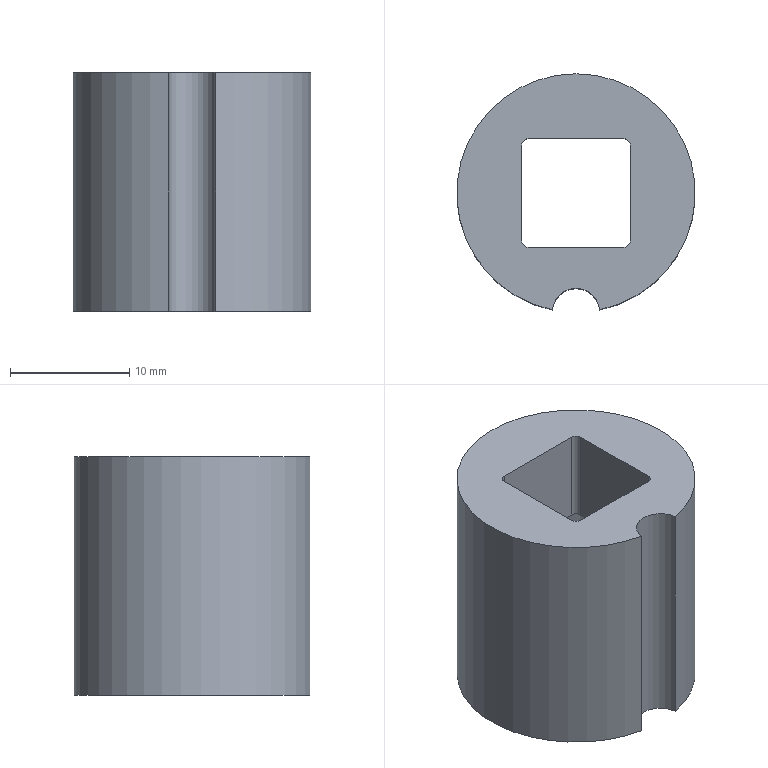Part | NX | features solid 2 | 1 solid | 14 faces | box 20 x 19.8 x 20 mm | volume 4006 mm3 | plane 7 | cylinder 7 | commonest cylinder face diameters 1.1 x4 4 x1 12.6 x1 20 x1
STEP:
#1=CARTESIAN_POINT('',(-513.119,-116.624,24.));
#2=VERTEX_POINT('',#1);
#3=CARTESIAN_POINT('',(-517.099,-116.624,24.));
#4=VERTEX_POINT('',#3);
#5=CARTESIAN_POINT('',(-515.109,-106.824,24.));
#6=DIRECTION('',(0.,0.,1.));
#7=DIRECTION('',(0.,-1.,0.));
#8=AXIS2_PLACEMENT_3D('',#5,#6,#7);
#9=CIRCLE('',#8,10.);
#10=EDGE_CURVE('',#2,#4,#9,.T.);
#11=ORIENTED_EDGE('',*,*,#10,.F.);
#12=CARTESIAN_POINT('',(-515.109,-116.824,24.));
#13=DIRECTION('',(0.,0.,1.));
#14=DIRECTION('',(0.,-1.,0.));
#15=AXIS2_PLACEMENT_3D('',#12,#13,#14);
#16=CIRCLE('',#15,2.);
#17=EDGE_CURVE('',#2,#4,#16,.T.);
#18=ORIENTED_EDGE('',*,*,#17,.T.);
#19=EDGE_LOOP('',(#11,#18));
#20=FACE_BOUND('',#19,.T.);
#21=CARTESIAN_POINT('',(-515.109,-113.124,24.));
#22=VERTEX_POINT('',#21);
#23=CARTESIAN_POINT('',(-515.109,-106.824,24.));
#24=DIRECTION('',(0.,0.,1.));
#25=DIRECTION('',(0.,-1.,0.));
#26=AXIS2_PLACEMENT_3D('',#23,#24,#25);
#27=CIRCLE('',#26,6.3);
#28=EDGE_CURVE('',#22,#22,#27,.T.);
#29=ORIENTED_EDGE('',*,*,#28,.T.);
#30=EDGE_LOOP('',(#29));
#31=FACE_BOUND('',#30,.T.);
#32=CARTESIAN_POINT('',(-515.109,-106.824,24.));
#33=DIRECTION('',(0.,0.,1.));
#34=DIRECTION('',(0.,-1.,0.));
#35=AXIS2_PLACEMENT_3D('',#32,#33,#34);
#36=PLANE('',#35);
#37=ADVANCED_FACE('',(#20,#31),#36,.F.);
#38=ORIENTED_EDGE('',*,*,#28,.F.);
#39=EDGE_LOOP('',(#38));
#40=FACE_BOUND('',#39,.T.);
#41=CARTESIAN_POINT('',(-515.109,-113.124,36.));
#42=VERTEX_POINT('',#41);
#43=CARTESIAN_POINT('',(-515.109,-106.824,36.));
#44=DIRECTION('',(0.,0.,1.));
#45=DIRECTION('',(0.,-1.,0.));
#46=AXIS2_PLACEMENT_3D('',#43,#44,#45);
#47=CIRCLE('',#46,6.3);
#48=EDGE_CURVE('',#42,#42,#47,.T.);
#49=ORIENTED_EDGE('',*,*,#48,.T.);
#50=EDGE_LOOP('',(#49));
#51=FACE_BOUND('',#50,.T.);
#52=CARTESIAN_POINT('',(-515.109,-106.824,24.));
#53=DIRECTION('',(0.,0.,1.));
#54=DIRECTION('',(0.,-1.,0.));
#55=AXIS2_PLACEMENT_3D('',#52,#53,#54);
#56=CYLINDRICAL_SURFACE('',#55,6.3);
#57=ADVANCED_FACE('',(#40,#51),#56,.F.);
#58=ORIENTED_EDGE('',*,*,#48,.F.);
#59=EDGE_LOOP('',(#58));
#60=FACE_BOUND('',#59,.T.);
#61=CARTESIAN_POINT('',(-510.559,-110.824,36.));
#62=VERTEX_POINT('',#61);
#63=CARTESIAN_POINT('',(-510.559,-102.824,36.));
#64=VERTEX_POINT('',#63);
#65=CARTESIAN_POINT('',(-510.559,-106.824,36.));
#66=DIRECTION('',(0.,1.,0.));
#67=VECTOR('',#66,1000.);
#68=LINE('',#65,#67);
#69=EDGE_CURVE('',#62,#64,#68,.T.);
#70=ORIENTED_EDGE('',*,*,#69,.T.);
#71=CARTESIAN_POINT('',(-511.109,-102.274,36.));
#72=VERTEX_POINT('',#71);
#73=CARTESIAN_POINT('',(-511.109,-102.824,36.));
#74=DIRECTION('',(0.,0.,1.));
#75=DIRECTION('',(0.,-1.,0.));
#76=AXIS2_PLACEMENT_3D('',#73,#74,#75);
#77=CIRCLE('',#76,0.55);
#78=EDGE_CURVE('',#64,#72,#77,.T.);
#79=ORIENTED_EDGE('',*,*,#78,.T.);
#80=CARTESIAN_POINT('',(-519.109,-102.274,36.));
#81=VERTEX_POINT('',#80);
#82=CARTESIAN_POINT('',(-515.109,-102.274,36.));
#83=DIRECTION('',(-1.,0.,0.));
#84=VECTOR('',#83,1000.);
#85=LINE('',#82,#84);
#86=EDGE_CURVE('',#72,#81,#85,.T.);
#87=ORIENTED_EDGE('',*,*,#86,.T.);
#88=CARTESIAN_POINT('',(-519.659,-102.824,36.));
#89=VERTEX_POINT('',#88);
#90=CARTESIAN_POINT('',(-519.109,-102.824,36.));
#91=DIRECTION('',(0.,0.,1.));
#92=DIRECTION('',(0.,-1.,0.));
#93=AXIS2_PLACEMENT_3D('',#90,#91,#92);
#94=CIRCLE('',#93,0.55);
#95=EDGE_CURVE('',#81,#89,#94,.T.);
#96=ORIENTED_EDGE('',*,*,#95,.T.);
#97=CARTESIAN_POINT('',(-519.659,-110.824,36.));
#98=VERTEX_POINT('',#97);
#99=CARTESIAN_POINT('',(-519.659,-106.824,36.));
#100=DIRECTION('',(0.,-1.,0.));
#101=VECTOR('',#100,1000.);
#102=LINE('',#99,#101);
#103=EDGE_CURVE('',#89,#98,#102,.T.);
#104=ORIENTED_EDGE('',*,*,#103,.T.);
#105=CARTESIAN_POINT('',(-519.109,-111.374,36.));
#106=VERTEX_POINT('',#105);
#107=CARTESIAN_POINT('',(-519.109,-110.824,36.));
#108=DIRECTION('',(0.,0.,1.));
#109=DIRECTION('',(0.,-1.,0.));
#110=AXIS2_PLACEMENT_3D('',#107,#108,#109);
#111=CIRCLE('',#110,0.55);
#112=EDGE_CURVE('',#98,#106,#111,.T.);
#113=ORIENTED_EDGE('',*,*,#112,.T.);
#114=CARTESIAN_POINT('',(-511.109,-111.374,36.));
#115=VERTEX_POINT('',#114);
#116=CARTESIAN_POINT('',(-515.109,-111.374,36.));
#117=DIRECTION('',(-1.,0.,0.));
#118=VECTOR('',#117,1000.);
#119=LINE('',#116,#118);
#120=EDGE_CURVE('',#115,#106,#119,.T.);
#121=ORIENTED_EDGE('',*,*,#120,.F.);
#122=CARTESIAN_POINT('',(-511.109,-110.824,36.));
#123=DIRECTION('',(0.,0.,1.));
#124=DIRECTION('',(0.,-1.,0.));
#125=AXIS2_PLACEMENT_3D('',#122,#123,#124);
#126=CIRCLE('',#125,0.55);
#127=EDGE_CURVE('',#115,#62,#126,.T.);
#128=ORIENTED_EDGE('',*,*,#127,.T.);
#129=EDGE_LOOP('',(#70,#79,#87,#96,#104,#113,#121,#128));
#130=FACE_BOUND('',#129,.T.);
#131=CARTESIAN_POINT('',(-515.109,-106.824,36.));
#132=DIRECTION('',(0.,0.,1.));
#133=DIRECTION('',(0.,-1.,0.));
#134=AXIS2_PLACEMENT_3D('',#131,#132,#133);
#135=PLANE('',#134);
#136=ADVANCED_FACE('',(#60,#130),#135,.F.);
#137=CARTESIAN_POINT('',(-513.119,-116.624,44.));
#138=VERTEX_POINT('',#137);
#139=CARTESIAN_POINT('',(-513.119,-116.624,34.));
#140=DIRECTION('',(0.,0.,1.));
#141=VECTOR('',#140,1000.);
#142=LINE('',#139,#141);
#143=EDGE_CURVE('',#2,#138,#142,.T.);
#144=ORIENTED_EDGE('',*,*,#143,.F.);
#145=ORIENTED_EDGE('',*,*,#10,.T.);
#146=CARTESIAN_POINT('',(-517.099,-116.624,44.));
#147=VERTEX_POINT('',#146);
#148=CARTESIAN_POINT('',(-517.099,-116.624,34.));
#149=DIRECTION('',(0.,0.,1.));
#150=VECTOR('',#149,1000.);
#151=LINE('',#148,#150);
#152=EDGE_CURVE('',#147,#4,#151,.F.);
#153=ORIENTED_EDGE('',*,*,#152,.F.);
#154=CARTESIAN_POINT('',(-515.109,-106.824,44.));
#155=DIRECTION('',(0.,0.,1.));
#156=DIRECTION('',(0.,-1.,0.));
#157=AXIS2_PLACEMENT_3D('',#154,#155,#156);
#158=CIRCLE('',#157,10.);
#159=EDGE_CURVE('',#138,#147,#158,.T.);
#160=ORIENTED_EDGE('',*,*,#159,.F.);
#161=EDGE_LOOP('',(#144,#145,#153,#160));
#162=FACE_BOUND('',#161,.T.);
#163=CARTESIAN_POINT('',(-515.109,-106.824,24.));
#164=DIRECTION('',(0.,0.,1.));
#165=DIRECTION('',(0.,-1.,0.));
#166=AXIS2_PLACEMENT_3D('',#163,#164,#165);
#167=CYLINDRICAL_SURFACE('',#166,10.);
#168=ADVANCED_FACE('',(#162),#167,.T.);
#169=CARTESIAN_POINT('',(-511.109,-102.274,44.));
#170=VERTEX_POINT('',#169);
#171=CARTESIAN_POINT('',(-519.109,-102.274,44.));
#172=VERTEX_POINT('',#171);
#173=CARTESIAN_POINT('',(-510.559,-102.274,44.));
#174=DIRECTION('',(-1.,0.,0.));
#175=VECTOR('',#174,1000.);
#176=LINE('',#173,#175);
#177=EDGE_CURVE('',#170,#172,#176,.T.);
#178=ORIENTED_EDGE('',*,*,#177,.F.);
#179=CARTESIAN_POINT('',(-510.559,-102.824,44.));
#180=VERTEX_POINT('',#179);
#181=CARTESIAN_POINT('',(-511.109,-102.824,44.));
#182=DIRECTION('',(0.,0.,1.));
#183=DIRECTION('',(0.,-1.,0.));
#184=AXIS2_PLACEMENT_3D('',#181,#182,#183);
#185=CIRCLE('',#184,0.55);
#186=EDGE_CURVE('',#170,#180,#185,.F.);
#187=ORIENTED_EDGE('',*,*,#186,.T.);
#188=CARTESIAN_POINT('',(-510.559,-110.824,44.));
#189=VERTEX_POINT('',#188);
#190=CARTESIAN_POINT('',(-510.559,-111.374,44.));
#191=DIRECTION('',(0.,1.,0.));
#192=VECTOR('',#191,1000.);
#193=LINE('',#190,#192);
#194=EDGE_CURVE('',#189,#180,#193,.T.);
#195=ORIENTED_EDGE('',*,*,#194,.F.);
#196=CARTESIAN_POINT('',(-511.109,-111.374,44.));
#197=VERTEX_POINT('',#196);
#198=CARTESIAN_POINT('',(-511.109,-110.824,44.));
#199=DIRECTION('',(0.,0.,1.));
#200=DIRECTION('',(0.,-1.,0.));
#201=AXIS2_PLACEMENT_3D('',#198,#199,#200);
#202=CIRCLE('',#201,0.55);
#203=EDGE_CURVE('',#189,#197,#202,.F.);
#204=ORIENTED_EDGE('',*,*,#203,.T.);
#205=CARTESIAN_POINT('',(-519.109,-111.374,44.));
#206=VERTEX_POINT('',#205);
#207=CARTESIAN_POINT('',(-510.559,-111.374,44.));
#208=DIRECTION('',(-1.,0.,0.));
#209=VECTOR('',#208,1000.);
#210=LINE('',#207,#209);
#211=EDGE_CURVE('',#197,#206,#210,.T.);
#212=ORIENTED_EDGE('',*,*,#211,.T.);
#213=CARTESIAN_POINT('',(-519.659,-110.824,44.));
#214=VERTEX_POINT('',#213);
#215=CARTESIAN_POINT('',(-519.109,-110.824,44.));
#216=DIRECTION('',(0.,0.,1.));
#217=DIRECTION('',(0.,-1.,0.));
#218=AXIS2_PLACEMENT_3D('',#215,#216,#217);
#219=CIRCLE('',#218,0.55);
#220=EDGE_CURVE('',#206,#214,#219,.F.);
#221=ORIENTED_EDGE('',*,*,#220,.T.);
#222=CARTESIAN_POINT('',(-519.659,-102.824,44.));
#223=VERTEX_POINT('',#222);
#224=CARTESIAN_POINT('',(-519.659,-102.274,44.));
#225=DIRECTION('',(0.,-1.,0.));
#226=VECTOR('',#225,1000.);
#227=LINE('',#224,#226);
#228=EDGE_CURVE('',#223,#214,#227,.T.);
#229=ORIENTED_EDGE('',*,*,#228,.F.);
#230=CARTESIAN_POINT('',(-519.109,-102.824,44.));
#231=DIRECTION('',(0.,0.,1.));
#232=DIRECTION('',(0.,-1.,0.));
#233=AXIS2_PLACEMENT_3D('',#230,#231,#232);
#234=CIRCLE('',#233,0.55);
#235=EDGE_CURVE('',#223,#172,#234,.F.);
#236=ORIENTED_EDGE('',*,*,#235,.T.);
#237=EDGE_LOOP('',(#178,#187,#195,#204,#212,#221,#229,#236));
#238=FACE_BOUND('',#237,.T.);
#239=CARTESIAN_POINT('',(-515.109,-116.824,44.));
#240=DIRECTION('',(0.,0.,1.));
#241=DIRECTION('',(0.,-1.,0.));
#242=AXIS2_PLACEMENT_3D('',#239,#240,#241);
#243=CIRCLE('',#242,2.);
#244=EDGE_CURVE('',#138,#147,#243,.T.);
#245=ORIENTED_EDGE('',*,*,#244,.F.);
#246=ORIENTED_EDGE('',*,*,#159,.T.);
#247=EDGE_LOOP('',(#245,#246));
#248=FACE_BOUND('',#247,.T.);
#249=CARTESIAN_POINT('',(-515.109,-106.824,44.));
#250=DIRECTION('',(0.,0.,1.));
#251=DIRECTION('',(0.,-1.,0.));
#252=AXIS2_PLACEMENT_3D('',#249,#250,#251);
#253=PLANE('',#252);
#254=ADVANCED_FACE('',(#238,#248),#253,.T.);
#255=ORIENTED_EDGE('',*,*,#143,.T.);
#256=ORIENTED_EDGE('',*,*,#244,.T.);
#257=ORIENTED_EDGE('',*,*,#152,.T.);
#258=ORIENTED_EDGE('',*,*,#17,.F.);
#259=EDGE_LOOP('',(#255,#256,#257,#258));
#260=FACE_BOUND('',#259,.T.);
#261=CARTESIAN_POINT('',(-515.109,-116.824,24.));
#262=DIRECTION('',(0.,0.,1.));
#263=DIRECTION('',(0.,-1.,0.));
#264=AXIS2_PLACEMENT_3D('',#261,#262,#263);
#265=CYLINDRICAL_SURFACE('',#264,2.);
#266=ADVANCED_FACE('',(#260),#265,.F.);
#267=ORIENTED_EDGE('',*,*,#177,.T.);
#268=CARTESIAN_POINT('',(-519.109,-102.274,24.));
#269=DIRECTION('',(0.,0.,1.));
#270=VECTOR('',#269,1000.);
#271=LINE('',#268,#270);
#272=EDGE_CURVE('',#172,#81,#271,.F.);
#273=ORIENTED_EDGE('',*,*,#272,.T.);
#274=ORIENTED_EDGE('',*,*,#86,.F.);
#275=CARTESIAN_POINT('',(-511.109,-102.274,44.));
#276=DIRECTION('',(0.,0.,1.));
#277=VECTOR('',#276,1000.);
#278=LINE('',#275,#277);
#279=EDGE_CURVE('',#72,#170,#278,.T.);
#280=ORIENTED_EDGE('',*,*,#279,.T.);
#281=EDGE_LOOP('',(#267,#273,#274,#280));
#282=FACE_BOUND('',#281,.T.);
#283=CARTESIAN_POINT('',(-510.559,-102.274,24.));
#284=DIRECTION('',(0.,1.,0.));
#285=DIRECTION('',(0.,0.,1.));
#286=AXIS2_PLACEMENT_3D('',#283,#284,#285);
#287=PLANE('',#286);
#288=ADVANCED_FACE('',(#282),#287,.F.);
#289=ORIENTED_EDGE('',*,*,#228,.T.);
#290=CARTESIAN_POINT('',(-519.659,-110.824,24.));
#291=DIRECTION('',(0.,0.,1.));
#292=VECTOR('',#291,1000.);
#293=LINE('',#290,#292);
#294=EDGE_CURVE('',#214,#98,#293,.F.);
#295=ORIENTED_EDGE('',*,*,#294,.T.);
#296=ORIENTED_EDGE('',*,*,#103,.F.);
#297=CARTESIAN_POINT('',(-519.659,-102.824,44.));
#298=DIRECTION('',(0.,0.,1.));
#299=VECTOR('',#298,1000.);
#300=LINE('',#297,#299);
#301=EDGE_CURVE('',#89,#223,#300,.T.);
#302=ORIENTED_EDGE('',*,*,#301,.T.);
#303=EDGE_LOOP('',(#289,#295,#296,#302));
#304=FACE_BOUND('',#303,.T.);
#305=CARTESIAN_POINT('',(-519.659,-102.274,24.));
#306=DIRECTION('',(-1.,0.,0.));
#307=DIRECTION('',(0.,0.,-1.));
#308=AXIS2_PLACEMENT_3D('',#305,#306,#307);
#309=PLANE('',#308);
#310=ADVANCED_FACE('',(#304),#309,.F.);
#311=ORIENTED_EDGE('',*,*,#211,.F.);
#312=CARTESIAN_POINT('',(-511.109,-111.374,24.));
#313=DIRECTION('',(0.,0.,1.));
#314=VECTOR('',#313,1000.);
#315=LINE('',#312,#314);
#316=EDGE_CURVE('',#197,#115,#315,.F.);
#317=ORIENTED_EDGE('',*,*,#316,.T.);
#318=ORIENTED_EDGE('',*,*,#120,.T.);
#319=CARTESIAN_POINT('',(-519.109,-111.374,24.));
#320=DIRECTION('',(0.,0.,1.));
#321=VECTOR('',#320,1000.);
#322=LINE('',#319,#321);
#323=EDGE_CURVE('',#106,#206,#322,.T.);
#324=ORIENTED_EDGE('',*,*,#323,.T.);
#325=EDGE_LOOP('',(#311,#317,#318,#324));
#326=FACE_BOUND('',#325,.T.);
#327=CARTESIAN_POINT('',(-510.559,-111.374,24.));
#328=DIRECTION('',(0.,1.,0.));
#329=DIRECTION('',(0.,0.,1.));
#330=AXIS2_PLACEMENT_3D('',#327,#328,#329);
#331=PLANE('',#330);
#332=ADVANCED_FACE('',(#326),#331,.T.);
#333=ORIENTED_EDGE('',*,*,#69,.F.);
#334=CARTESIAN_POINT('',(-510.559,-110.824,24.));
#335=DIRECTION('',(0.,0.,1.));
#336=VECTOR('',#335,1000.);
#337=LINE('',#334,#336);
#338=EDGE_CURVE('',#62,#189,#337,.T.);
#339=ORIENTED_EDGE('',*,*,#338,.T.);
#340=ORIENTED_EDGE('',*,*,#194,.T.);
#341=CARTESIAN_POINT('',(-510.559,-102.824,24.));
#342=DIRECTION('',(0.,0.,1.));
#343=VECTOR('',#342,1000.);
#344=LINE('',#341,#343);
#345=EDGE_CURVE('',#180,#64,#344,.F.);
#346=ORIENTED_EDGE('',*,*,#345,.T.);
#347=EDGE_LOOP('',(#333,#339,#340,#346));
#348=FACE_BOUND('',#347,.T.);
#349=CARTESIAN_POINT('',(-510.559,-111.374,24.));
#350=DIRECTION('',(1.,0.,0.));
#351=DIRECTION('',(0.,0.,1.));
#352=AXIS2_PLACEMENT_3D('',#349,#350,#351);
#353=PLANE('',#352);
#354=ADVANCED_FACE('',(#348),#353,.F.);
#355=ORIENTED_EDGE('',*,*,#127,.F.);
#356=ORIENTED_EDGE('',*,*,#316,.F.);
#357=ORIENTED_EDGE('',*,*,#203,.F.);
#358=ORIENTED_EDGE('',*,*,#338,.F.);
#359=EDGE_LOOP('',(#355,#356,#357,#358));
#360=FACE_BOUND('',#359,.T.);
#361=CARTESIAN_POINT('',(-511.109,-110.824,24.));
#362=DIRECTION('',(0.,0.,1.));
#363=DIRECTION('',(0.,-1.,0.));
#364=AXIS2_PLACEMENT_3D('',#361,#362,#363);
#365=CYLINDRICAL_SURFACE('',#364,0.55);
#366=ADVANCED_FACE('',(#360),#365,.F.);
#367=ORIENTED_EDGE('',*,*,#112,.F.);
#368=ORIENTED_EDGE('',*,*,#294,.F.);
#369=ORIENTED_EDGE('',*,*,#220,.F.);
#370=ORIENTED_EDGE('',*,*,#323,.F.);
#371=EDGE_LOOP('',(#367,#368,#369,#370));
#372=FACE_BOUND('',#371,.T.);
#373=CARTESIAN_POINT('',(-519.109,-110.824,24.));
#374=DIRECTION('',(0.,0.,1.));
#375=DIRECTION('',(0.,-1.,0.));
#376=AXIS2_PLACEMENT_3D('',#373,#374,#375);
#377=CYLINDRICAL_SURFACE('',#376,0.55);
#378=ADVANCED_FACE('',(#372),#377,.F.);
#379=ORIENTED_EDGE('',*,*,#95,.F.);
#380=ORIENTED_EDGE('',*,*,#272,.F.);
#381=ORIENTED_EDGE('',*,*,#235,.F.);
#382=ORIENTED_EDGE('',*,*,#301,.F.);
#383=EDGE_LOOP('',(#379,#380,#381,#382));
#384=FACE_BOUND('',#383,.T.);
#385=CARTESIAN_POINT('',(-519.109,-102.824,24.));
#386=DIRECTION('',(0.,0.,-1.));
#387=DIRECTION('',(0.,1.,0.));
#388=AXIS2_PLACEMENT_3D('',#385,#386,#387);
#389=CYLINDRICAL_SURFACE('',#388,0.55);
#390=ADVANCED_FACE('',(#384),#389,.F.);
#391=ORIENTED_EDGE('',*,*,#78,.F.);
#392=ORIENTED_EDGE('',*,*,#345,.F.);
#393=ORIENTED_EDGE('',*,*,#186,.F.);
#394=ORIENTED_EDGE('',*,*,#279,.F.);
#395=EDGE_LOOP('',(#391,#392,#393,#394));
#396=FACE_BOUND('',#395,.T.);
#397=CARTESIAN_POINT('',(-511.109,-102.824,24.));
#398=DIRECTION('',(0.,0.,-1.));
#399=DIRECTION('',(0.,1.,0.));
#400=AXIS2_PLACEMENT_3D('',#397,#398,#399);
#401=CYLINDRICAL_SURFACE('',#400,0.55);
#402=ADVANCED_FACE('',(#396),#401,.F.);
#403=CLOSED_SHELL('',(#37,#57,#136,#168,#254,#266,#288,#310,#332,#354,#366,#378,#390,#402));
#404=MANIFOLD_SOLID_BREP('',#403);
#405=(LENGTH_UNIT()NAMED_UNIT(*)SI_UNIT(.MILLI.,.METRE.));
#406=UNCERTAINTY_MEASURE_WITH_UNIT(LENGTH_MEASURE(0.00001),#405,'','');
#407=(NAMED_UNIT(*)PLANE_ANGLE_UNIT()SI_UNIT($,.RADIAN.));
#408=(NAMED_UNIT(*)SI_UNIT($,.STERADIAN.)SOLID_ANGLE_UNIT());
#409=(GEOMETRIC_REPRESENTATION_CONTEXT(3)GLOBAL_UNCERTAINTY_ASSIGNED_CONTEXT((#406))GLOBAL_UNIT_ASSIGNED_CONTEXT((#405,#407,#408))REPRESENTATION_CONTEXT('',''));
#410=ADVANCED_BREP_SHAPE_REPRESENTATION('',(#404),#409);